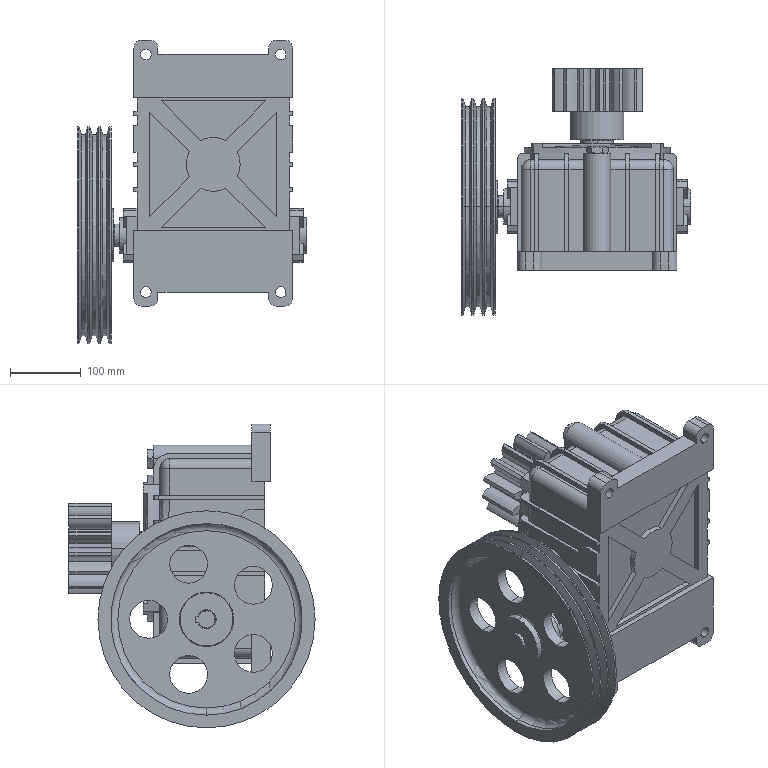Part | SolidWorks | features CompositeCurve 1 | 5 solids | 676 faces | box 324 x 347 x 428.15 mm | volume 12606239 mm3 | plane 352 | cylinder 203 | cone 55 | spline 34 | torus 28 | sphere 4 | commonest cylinder face diameters 28.125 x20 7.268 x16 7.65 x16 92 x14 128 x14 53.3 x10